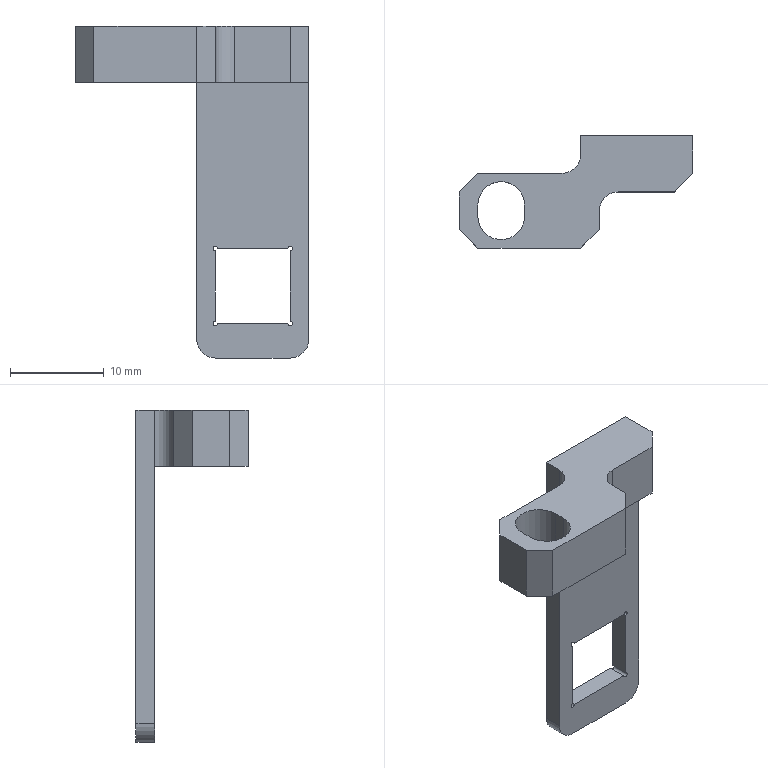Part | SolidWorks | features ICE 7, Fillet 2, 3DProfileFeature 1, Chamfer 1, Extrusion 1, HoleWzd 1 | 1 solid | 34 faces | box 25 x 12 x 35.5 mm | volume 1512 mm3 | plane 22 | cylinder 12 | commonest cylinder face diameters 0.5 x6 4 x4 5 x2
STEP:
#1=CARTESIAN_POINT('',(4.,0.,-9.8));
#2=VERTEX_POINT('',#1);
#3=CARTESIAN_POINT('',(4.,0.,-10.3));
#4=VERTEX_POINT('',#3);
#5=CARTESIAN_POINT('',(4.,0.,-10.05));
#6=DIRECTION('',(0.,1.,0.));
#7=DIRECTION('',(0.,0.,1.));
#8=AXIS2_PLACEMENT_3D('',#5,#6,#7);
#9=CIRCLE('',#8,0.25);
#10=EDGE_CURVE('',#2,#4,#9,.T.);
#11=ORIENTED_EDGE('',*,*,#10,.F.);
#12=CARTESIAN_POINT('',(4.,2.,-9.8));
#13=VERTEX_POINT('',#12);
#14=CARTESIAN_POINT('',(4.,-8.,-9.8));
#15=DIRECTION('',(0.,1.,0.));
#16=VECTOR('',#15,1000.);
#17=LINE('',#14,#16);
#18=EDGE_CURVE('',#2,#13,#17,.T.);
#19=ORIENTED_EDGE('',*,*,#18,.T.);
#20=CARTESIAN_POINT('',(4.,2.,-10.3));
#21=VERTEX_POINT('',#20);
#22=CARTESIAN_POINT('',(4.,2.,-10.05));
#23=DIRECTION('',(0.,1.,0.));
#24=DIRECTION('',(0.,0.,1.));
#25=AXIS2_PLACEMENT_3D('',#22,#23,#24);
#26=CIRCLE('',#25,0.25);
#27=EDGE_CURVE('',#13,#21,#26,.T.);
#28=ORIENTED_EDGE('',*,*,#27,.T.);
#29=CARTESIAN_POINT('',(4.,-8.,-10.3));
#30=DIRECTION('',(0.,1.,0.));
#31=VECTOR('',#30,1000.);
#32=LINE('',#29,#31);
#33=EDGE_CURVE('',#4,#21,#32,.T.);
#34=ORIENTED_EDGE('',*,*,#33,.F.);
#35=EDGE_LOOP('',(#11,#19,#28,#34));
#36=FACE_OUTER_BOUND('',#35,.T.);
#37=CARTESIAN_POINT('',(4.,-8.,-10.05));
#38=DIRECTION('',(0.,1.,0.));
#39=DIRECTION('',(0.,0.,1.));
#40=AXIS2_PLACEMENT_3D('',#37,#38,#39);
#41=CYLINDRICAL_SURFACE('',#40,0.25);
#42=ADVANCED_FACE('',(#36),#41,.F.);
#43=CARTESIAN_POINT('',(-4.,0.,-9.8));
#44=VERTEX_POINT('',#43);
#45=CARTESIAN_POINT('',(-3.75,0.,-10.05));
#46=VERTEX_POINT('',#45);
#47=CARTESIAN_POINT('',(-4.,0.,-10.05));
#48=DIRECTION('',(0.,1.,0.));
#49=DIRECTION('',(0.,0.,1.));
#50=AXIS2_PLACEMENT_3D('',#47,#48,#49);
#51=CIRCLE('',#50,0.25);
#52=EDGE_CURVE('',#44,#46,#51,.T.);
#53=ORIENTED_EDGE('',*,*,#52,.F.);
#54=CARTESIAN_POINT('',(-4.,2.,-9.8));
#55=VERTEX_POINT('',#54);
#56=CARTESIAN_POINT('',(-4.,-8.,-9.8));
#57=DIRECTION('',(0.,1.,0.));
#58=VECTOR('',#57,1000.);
#59=LINE('',#56,#58);
#60=EDGE_CURVE('',#44,#55,#59,.T.);
#61=ORIENTED_EDGE('',*,*,#60,.T.);
#62=CARTESIAN_POINT('',(-3.75,2.,-10.05));
#63=VERTEX_POINT('',#62);
#64=CARTESIAN_POINT('',(-4.,2.,-10.05));
#65=DIRECTION('',(0.,1.,0.));
#66=DIRECTION('',(0.,0.,1.));
#67=AXIS2_PLACEMENT_3D('',#64,#65,#66);
#68=CIRCLE('',#67,0.25);
#69=EDGE_CURVE('',#55,#63,#68,.T.);
#70=ORIENTED_EDGE('',*,*,#69,.T.);
#71=CARTESIAN_POINT('',(-3.75,-8.,-10.05));
#72=DIRECTION('',(0.,1.,0.));
#73=VECTOR('',#72,1000.);
#74=LINE('',#71,#73);
#75=EDGE_CURVE('',#46,#63,#74,.T.);
#76=ORIENTED_EDGE('',*,*,#75,.F.);
#77=EDGE_LOOP('',(#53,#61,#70,#76));
#78=FACE_OUTER_BOUND('',#77,.T.);
#79=CARTESIAN_POINT('',(-4.,-8.,-10.05));
#80=DIRECTION('',(0.,1.,0.));
#81=DIRECTION('',(0.,0.,1.));
#82=AXIS2_PLACEMENT_3D('',#79,#80,#81);
#83=CYLINDRICAL_SURFACE('',#82,0.25);
#84=ADVANCED_FACE('',(#78),#83,.F.);
#85=CARTESIAN_POINT('',(6.,0.,7.75));
#86=VERTEX_POINT('',#85);
#87=CARTESIAN_POINT('',(6.,0.,-19.75));
#88=VERTEX_POINT('',#87);
#89=CARTESIAN_POINT('',(6.,0.,-21.75));
#90=DIRECTION('',(0.,0.,-1.));
#91=VECTOR('',#90,1000.);
#92=LINE('',#89,#91);
#93=EDGE_CURVE('',#86,#88,#92,.T.);
#94=ORIENTED_EDGE('',*,*,#93,.T.);
#95=CARTESIAN_POINT('',(6.,2.,-19.75));
#96=VERTEX_POINT('',#95);
#97=CARTESIAN_POINT('',(6.,2.,-19.75));
#98=DIRECTION('',(0.,1.,0.));
#99=VECTOR('',#98,1000.);
#100=LINE('',#97,#99);
#101=EDGE_CURVE('',#88,#96,#100,.T.);
#102=ORIENTED_EDGE('',*,*,#101,.T.);
#103=CARTESIAN_POINT('',(6.,2.,13.75));
#104=VERTEX_POINT('',#103);
#105=CARTESIAN_POINT('',(6.,2.,-21.75));
#106=DIRECTION('',(0.,0.,-1.));
#107=VECTOR('',#106,1000.);
#108=LINE('',#105,#107);
#109=EDGE_CURVE('',#104,#96,#108,.T.);
#110=ORIENTED_EDGE('',*,*,#109,.F.);
#111=CARTESIAN_POINT('',(6.,-2.,13.75));
#112=VERTEX_POINT('',#111);
#113=CARTESIAN_POINT('',(6.,-10.,13.75));
#114=DIRECTION('',(0.,1.,0.));
#115=VECTOR('',#114,1000.);
#116=LINE('',#113,#115);
#117=EDGE_CURVE('',#112,#104,#116,.T.);
#118=ORIENTED_EDGE('',*,*,#117,.F.);
#119=CARTESIAN_POINT('',(6.,-2.,7.75));
#120=VERTEX_POINT('',#119);
#121=CARTESIAN_POINT('',(6.,-2.,-21.75));
#122=DIRECTION('',(0.,0.,-1.));
#123=VECTOR('',#122,1000.);
#124=LINE('',#121,#123);
#125=EDGE_CURVE('',#112,#120,#124,.T.);
#126=ORIENTED_EDGE('',*,*,#125,.T.);
#127=CARTESIAN_POINT('',(6.,2.,7.75));
#128=DIRECTION('',(0.,1.,0.));
#129=VECTOR('',#128,1000.);
#130=LINE('',#127,#129);
#131=EDGE_CURVE('',#120,#86,#130,.T.);
#132=ORIENTED_EDGE('',*,*,#131,.T.);
#133=EDGE_LOOP('',(#94,#102,#110,#118,#126,#132));
#134=FACE_OUTER_BOUND('',#133,.T.);
#135=CARTESIAN_POINT('',(6.,2.,-21.75));
#136=DIRECTION('',(-1.,0.,0.));
#137=DIRECTION('',(0.,0.,1.));
#138=AXIS2_PLACEMENT_3D('',#135,#136,#137);
#139=PLANE('',#138);
#140=ADVANCED_FACE('',(#134),#139,.F.);
#141=CARTESIAN_POINT('',(4.,2.,-21.75));
#142=VERTEX_POINT('',#141);
#143=CARTESIAN_POINT('',(-4.,2.,-21.75));
#144=VERTEX_POINT('',#143);
#145=CARTESIAN_POINT('',(-6.,2.,-21.75));
#146=DIRECTION('',(-1.,0.,0.));
#147=VECTOR('',#146,1000.);
#148=LINE('',#145,#147);
#149=EDGE_CURVE('',#142,#144,#148,.T.);
#150=ORIENTED_EDGE('',*,*,#149,.F.);
#151=CARTESIAN_POINT('',(4.,0.,-21.75));
#152=VERTEX_POINT('',#151);
#153=CARTESIAN_POINT('',(4.,2.,-21.75));
#154=DIRECTION('',(0.,-1.,0.));
#155=VECTOR('',#154,1000.);
#156=LINE('',#153,#155);
#157=EDGE_CURVE('',#142,#152,#156,.T.);
#158=ORIENTED_EDGE('',*,*,#157,.T.);
#159=CARTESIAN_POINT('',(-4.,0.,-21.75));
#160=VERTEX_POINT('',#159);
#161=CARTESIAN_POINT('',(-6.,0.,-21.75));
#162=DIRECTION('',(-1.,0.,0.));
#163=VECTOR('',#162,1000.);
#164=LINE('',#161,#163);
#165=EDGE_CURVE('',#152,#160,#164,.T.);
#166=ORIENTED_EDGE('',*,*,#165,.T.);
#167=CARTESIAN_POINT('',(-4.,2.,-21.75));
#168=DIRECTION('',(0.,1.,0.));
#169=VECTOR('',#168,1000.);
#170=LINE('',#167,#169);
#171=EDGE_CURVE('',#160,#144,#170,.T.);
#172=ORIENTED_EDGE('',*,*,#171,.T.);
#173=EDGE_LOOP('',(#150,#158,#166,#172));
#174=FACE_OUTER_BOUND('',#173,.T.);
#175=CARTESIAN_POINT('',(-6.,2.,-21.75));
#176=DIRECTION('',(0.,0.,1.));
#177=DIRECTION('',(1.,0.,0.));
#178=AXIS2_PLACEMENT_3D('',#175,#176,#177);
#179=PLANE('',#178);
#180=ADVANCED_FACE('',(#174),#179,.F.);
#181=CARTESIAN_POINT('',(-6.,2.,-19.75));
#182=VERTEX_POINT('',#181);
#183=CARTESIAN_POINT('',(-6.,2.,13.75));
#184=VERTEX_POINT('',#183);
#185=CARTESIAN_POINT('',(-6.,2.,-21.75));
#186=DIRECTION('',(0.,0.,1.));
#187=VECTOR('',#186,1000.);
#188=LINE('',#185,#187);
#189=EDGE_CURVE('',#182,#184,#188,.T.);
#190=ORIENTED_EDGE('',*,*,#189,.F.);
#191=CARTESIAN_POINT('',(-6.,0.,-19.75));
#192=VERTEX_POINT('',#191);
#193=CARTESIAN_POINT('',(-6.,2.,-19.75));
#194=DIRECTION('',(0.,-1.,0.));
#195=VECTOR('',#194,1000.);
#196=LINE('',#193,#195);
#197=EDGE_CURVE('',#182,#192,#196,.T.);
#198=ORIENTED_EDGE('',*,*,#197,.T.);
#199=CARTESIAN_POINT('',(-6.,0.,7.75));
#200=VERTEX_POINT('',#199);
#201=CARTESIAN_POINT('',(-6.,0.,-21.75));
#202=DIRECTION('',(0.,0.,1.));
#203=VECTOR('',#202,1000.);
#204=LINE('',#201,#203);
#205=EDGE_CURVE('',#192,#200,#204,.T.);
#206=ORIENTED_EDGE('',*,*,#205,.T.);
#207=CARTESIAN_POINT('',(-6.,0.,13.75));
#208=VERTEX_POINT('',#207);
#209=CARTESIAN_POINT('',(-6.,0.,13.75));
#210=DIRECTION('',(0.,0.,1.));
#211=VECTOR('',#210,1000.);
#212=LINE('',#209,#211);
#213=EDGE_CURVE('',#200,#208,#212,.T.);
#214=ORIENTED_EDGE('',*,*,#213,.T.);
#215=CARTESIAN_POINT('',(-6.,2.,13.75));
#216=DIRECTION('',(0.,1.,0.));
#217=VECTOR('',#216,1000.);
#218=LINE('',#215,#217);
#219=EDGE_CURVE('',#208,#184,#218,.T.);
#220=ORIENTED_EDGE('',*,*,#219,.T.);
#221=EDGE_LOOP('',(#190,#198,#206,#214,#220));
#222=FACE_OUTER_BOUND('',#221,.T.);
#223=CARTESIAN_POINT('',(-6.,2.,-21.75));
#224=DIRECTION('',(1.,0.,0.));
#225=DIRECTION('',(0.,0.,-1.));
#226=AXIS2_PLACEMENT_3D('',#223,#224,#225);
#227=PLANE('',#226);
#228=ADVANCED_FACE('',(#222),#227,.F.);
#229=CARTESIAN_POINT('',(4.,2.,-17.8));
#230=VERTEX_POINT('',#229);
#231=CARTESIAN_POINT('',(3.75,2.,-18.05));
#232=VERTEX_POINT('',#231);
#233=CARTESIAN_POINT('',(4.,2.,-18.05));
#234=DIRECTION('',(0.,1.,0.));
#235=DIRECTION('',(0.,0.,1.));
#236=AXIS2_PLACEMENT_3D('',#233,#234,#235);
#237=CIRCLE('',#236,0.25);
#238=EDGE_CURVE('',#230,#232,#237,.T.);
#239=ORIENTED_EDGE('',*,*,#238,.F.);
#240=CARTESIAN_POINT('',(4.,2.,-10.05));
#241=DIRECTION('',(0.,0.,-1.));
#242=VECTOR('',#241,1000.);
#243=LINE('',#240,#242);
#244=EDGE_CURVE('',#21,#230,#243,.T.);
#245=ORIENTED_EDGE('',*,*,#244,.F.);
#246=ORIENTED_EDGE('',*,*,#27,.F.);
#247=CARTESIAN_POINT('',(3.75,2.,-10.05));
#248=VERTEX_POINT('',#247);
#249=CARTESIAN_POINT('',(4.,2.,-10.05));
#250=DIRECTION('',(0.,1.,0.));
#251=DIRECTION('',(0.,0.,1.));
#252=AXIS2_PLACEMENT_3D('',#249,#250,#251);
#253=CIRCLE('',#252,0.25);
#254=EDGE_CURVE('',#248,#13,#253,.T.);
#255=ORIENTED_EDGE('',*,*,#254,.F.);
#256=CARTESIAN_POINT('',(-4.,2.,-10.05));
#257=DIRECTION('',(1.,0.,0.));
#258=VECTOR('',#257,1000.);
#259=LINE('',#256,#258);
#260=EDGE_CURVE('',#63,#248,#259,.T.);
#261=ORIENTED_EDGE('',*,*,#260,.F.);
#262=ORIENTED_EDGE('',*,*,#69,.F.);
#263=CARTESIAN_POINT('',(-4.,2.,-10.3));
#264=VERTEX_POINT('',#263);
#265=CARTESIAN_POINT('',(-4.,2.,-10.05));
#266=DIRECTION('',(0.,1.,0.));
#267=DIRECTION('',(0.,0.,1.));
#268=AXIS2_PLACEMENT_3D('',#265,#266,#267);
#269=CIRCLE('',#268,0.25);
#270=EDGE_CURVE('',#264,#55,#269,.T.);
#271=ORIENTED_EDGE('',*,*,#270,.F.);
#272=CARTESIAN_POINT('',(-4.,2.,-17.8));
#273=VERTEX_POINT('',#272);
#274=CARTESIAN_POINT('',(-4.,2.,-10.05));
#275=DIRECTION('',(0.,0.,1.));
#276=VECTOR('',#275,1000.);
#277=LINE('',#274,#276);
#278=EDGE_CURVE('',#273,#264,#277,.T.);
#279=ORIENTED_EDGE('',*,*,#278,.F.);
#280=CARTESIAN_POINT('',(-3.75,2.,-18.05));
#281=VERTEX_POINT('',#280);
#282=CARTESIAN_POINT('',(-4.,2.,-18.05));
#283=DIRECTION('',(0.,1.,0.));
#284=DIRECTION('',(0.,0.,1.));
#285=AXIS2_PLACEMENT_3D('',#282,#283,#284);
#286=CIRCLE('',#285,0.25);
#287=EDGE_CURVE('',#281,#273,#286,.T.);
#288=ORIENTED_EDGE('',*,*,#287,.F.);
#289=CARTESIAN_POINT('',(-4.,2.,-18.05));
#290=DIRECTION('',(-1.,0.,0.));
#291=VECTOR('',#290,1000.);
#292=LINE('',#289,#291);
#293=EDGE_CURVE('',#232,#281,#292,.T.);
#294=ORIENTED_EDGE('',*,*,#293,.F.);
#295=EDGE_LOOP('',(#239,#245,#246,#255,#261,#262,#271,#279,#288,#294));
#296=FACE_BOUND('',#295,.T.);
#297=ORIENTED_EDGE('',*,*,#109,.T.);
#298=CARTESIAN_POINT('',(4.,2.,-19.75));
#299=DIRECTION('',(0.,1.,0.));
#300=DIRECTION('',(0.,0.,1.));
#301=AXIS2_PLACEMENT_3D('',#298,#299,#300);
#302=CIRCLE('',#301,2.);
#303=EDGE_CURVE('',#96,#142,#302,.T.);
#304=ORIENTED_EDGE('',*,*,#303,.T.);
#305=ORIENTED_EDGE('',*,*,#149,.T.);
#306=CARTESIAN_POINT('',(-4.,2.,-19.75));
#307=DIRECTION('',(0.,1.,0.));
#308=DIRECTION('',(0.,0.,1.));
#309=AXIS2_PLACEMENT_3D('',#306,#307,#308);
#310=CIRCLE('',#309,2.);
#311=EDGE_CURVE('',#144,#182,#310,.T.);
#312=ORIENTED_EDGE('',*,*,#311,.T.);
#313=ORIENTED_EDGE('',*,*,#189,.T.);
#314=CARTESIAN_POINT('',(6.,2.,13.75));
#315=DIRECTION('',(-1.,0.,0.));
#316=VECTOR('',#315,1000.);
#317=LINE('',#314,#316);
#318=EDGE_CURVE('',#104,#184,#317,.T.);
#319=ORIENTED_EDGE('',*,*,#318,.F.);
#320=EDGE_LOOP('',(#297,#304,#305,#312,#313,#319));
#321=FACE_OUTER_BOUND('',#320,.T.);
#322=CARTESIAN_POINT('',(0.,2.,0.));
#323=DIRECTION('',(0.,1.,0.));
#324=DIRECTION('',(0.,0.,1.));
#325=AXIS2_PLACEMENT_3D('',#322,#323,#324);
#326=PLANE('',#325);
#327=ADVANCED_FACE('',(#296,#321),#326,.T.);
#328=CARTESIAN_POINT('',(4.,0.,-17.8));
#329=VERTEX_POINT('',#328);
#330=CARTESIAN_POINT('',(4.,0.,0.));
#331=DIRECTION('',(0.,0.,-1.));
#332=VECTOR('',#331,1000.);
#333=LINE('',#330,#332);
#334=EDGE_CURVE('',#4,#329,#333,.T.);
#335=ORIENTED_EDGE('',*,*,#334,.T.);
#336=CARTESIAN_POINT('',(3.75,0.,-18.05));
#337=VERTEX_POINT('',#336);
#338=CARTESIAN_POINT('',(4.,0.,-18.05));
#339=DIRECTION('',(0.,1.,0.));
#340=DIRECTION('',(0.,0.,1.));
#341=AXIS2_PLACEMENT_3D('',#338,#339,#340);
#342=CIRCLE('',#341,0.25);
#343=EDGE_CURVE('',#329,#337,#342,.T.);
#344=ORIENTED_EDGE('',*,*,#343,.T.);
#345=CARTESIAN_POINT('',(-3.75,0.,-18.05));
#346=VERTEX_POINT('',#345);
#347=CARTESIAN_POINT('',(0.,0.,-18.05));
#348=DIRECTION('',(-1.,0.,0.));
#349=VECTOR('',#348,1000.);
#350=LINE('',#347,#349);
#351=EDGE_CURVE('',#337,#346,#350,.T.);
#352=ORIENTED_EDGE('',*,*,#351,.T.);
#353=CARTESIAN_POINT('',(-4.,0.,-17.8));
#354=VERTEX_POINT('',#353);
#355=CARTESIAN_POINT('',(-4.,0.,-18.05));
#356=DIRECTION('',(0.,1.,0.));
#357=DIRECTION('',(0.,0.,1.));
#358=AXIS2_PLACEMENT_3D('',#355,#356,#357);
#359=CIRCLE('',#358,0.25);
#360=EDGE_CURVE('',#346,#354,#359,.T.);
#361=ORIENTED_EDGE('',*,*,#360,.T.);
#362=CARTESIAN_POINT('',(-4.,0.,-10.3));
#363=VERTEX_POINT('',#362);
#364=CARTESIAN_POINT('',(-4.,0.,0.));
#365=DIRECTION('',(0.,0.,1.));
#366=VECTOR('',#365,1000.);
#367=LINE('',#364,#366);
#368=EDGE_CURVE('',#354,#363,#367,.T.);
#369=ORIENTED_EDGE('',*,*,#368,.T.);
#370=CARTESIAN_POINT('',(-4.,0.,-10.05));
#371=DIRECTION('',(0.,1.,0.));
#372=DIRECTION('',(0.,0.,1.));
#373=AXIS2_PLACEMENT_3D('',#370,#371,#372);
#374=CIRCLE('',#373,0.25);
#375=EDGE_CURVE('',#363,#44,#374,.T.);
#376=ORIENTED_EDGE('',*,*,#375,.T.);
#377=ORIENTED_EDGE('',*,*,#52,.T.);
#378=CARTESIAN_POINT('',(3.75,0.,-10.05));
#379=VERTEX_POINT('',#378);
#380=CARTESIAN_POINT('',(0.,0.,-10.05));
#381=DIRECTION('',(1.,0.,0.));
#382=VECTOR('',#381,1000.);
#383=LINE('',#380,#382);
#384=EDGE_CURVE('',#46,#379,#383,.T.);
#385=ORIENTED_EDGE('',*,*,#384,.T.);
#386=CARTESIAN_POINT('',(4.,0.,-10.05));
#387=DIRECTION('',(0.,1.,0.));
#388=DIRECTION('',(0.,0.,1.));
#389=AXIS2_PLACEMENT_3D('',#386,#387,#388);
#390=CIRCLE('',#389,0.25);
#391=EDGE_CURVE('',#379,#2,#390,.T.);
#392=ORIENTED_EDGE('',*,*,#391,.T.);
#393=ORIENTED_EDGE('',*,*,#10,.T.);
#394=EDGE_LOOP('',(#335,#344,#352,#361,#369,#376,#377,#385,#392,#393));
#395=FACE_BOUND('',#394,.T.);
#396=ORIENTED_EDGE('',*,*,#165,.F.);
#397=CARTESIAN_POINT('',(4.,0.,-19.75));
#398=DIRECTION('',(0.,-1.,0.));
#399=DIRECTION('',(0.,0.,1.));
#400=AXIS2_PLACEMENT_3D('',#397,#398,#399);
#401=CIRCLE('',#400,2.);
#402=EDGE_CURVE('',#152,#88,#401,.T.);
#403=ORIENTED_EDGE('',*,*,#402,.T.);
#404=ORIENTED_EDGE('',*,*,#93,.F.);
#405=CARTESIAN_POINT('',(0.,0.,7.75));
#406=DIRECTION('',(-1.,0.,0.));
#407=VECTOR('',#406,1000.);
#408=LINE('',#405,#407);
#409=EDGE_CURVE('',#86,#200,#408,.T.);
#410=ORIENTED_EDGE('',*,*,#409,.T.);
#411=ORIENTED_EDGE('',*,*,#205,.F.);
#412=CARTESIAN_POINT('',(-4.,0.,-19.75));
#413=DIRECTION('',(0.,-1.,0.));
#414=DIRECTION('',(0.,0.,1.));
#415=AXIS2_PLACEMENT_3D('',#412,#413,#414);
#416=CIRCLE('',#415,2.);
#417=EDGE_CURVE('',#192,#160,#416,.T.);
#418=ORIENTED_EDGE('',*,*,#417,.T.);
#419=EDGE_LOOP('',(#396,#403,#404,#410,#411,#418));
#420=FACE_OUTER_BOUND('',#419,.T.);
#421=CARTESIAN_POINT('',(0.,0.,0.));
#422=DIRECTION('',(0.,1.,0.));
#423=DIRECTION('',(0.,0.,1.));
#424=AXIS2_PLACEMENT_3D('',#421,#422,#423);
#425=PLANE('',#424);
#426=ADVANCED_FACE('',(#395,#420),#425,.F.);
#427=CARTESIAN_POINT('',(-17.,-5.4,7.75));
#428=VERTEX_POINT('',#427);
#429=CARTESIAN_POINT('',(-12.,-5.4,7.75));
#430=VERTEX_POINT('',#429);
#431=CARTESIAN_POINT('',(-14.5,-5.4,7.75));
#432=DIRECTION('',(0.,0.,-1.));
#433=DIRECTION('',(-1.,0.,0.));
#434=AXIS2_PLACEMENT_3D('',#431,#432,#433);
#435=CIRCLE('',#434,2.5);
#436=EDGE_CURVE('',#428,#430,#435,.T.);
#437=ORIENTED_EDGE('',*,*,#436,.F.);
#438=CARTESIAN_POINT('',(-17.,-6.6,7.75));
#439=VERTEX_POINT('',#438);
#440=CARTESIAN_POINT('',(-17.,0.,7.75));
#441=DIRECTION('',(0.,1.,0.));
#442=VECTOR('',#441,1000.);
#443=LINE('',#440,#442);
#444=EDGE_CURVE('',#439,#428,#443,.T.);
#445=ORIENTED_EDGE('',*,*,#444,.F.);
#446=CARTESIAN_POINT('',(-12.,-6.6,7.75));
#447=VERTEX_POINT('',#446);
#448=CARTESIAN_POINT('',(-14.5,-6.6,7.75));
#449=DIRECTION('',(0.,0.,-1.));
#450=DIRECTION('',(-1.,0.,0.));
#451=AXIS2_PLACEMENT_3D('',#448,#449,#450);
#452=CIRCLE('',#451,2.5);
#453=EDGE_CURVE('',#447,#439,#452,.T.);
#454=ORIENTED_EDGE('',*,*,#453,.F.);
#455=CARTESIAN_POINT('',(-12.,0.,7.75));
#456=DIRECTION('',(0.,-1.,0.));
#457=VECTOR('',#456,1000.);
#458=LINE('',#455,#457);
#459=EDGE_CURVE('',#430,#447,#458,.T.);
#460=ORIENTED_EDGE('',*,*,#459,.F.);
#461=EDGE_LOOP('',(#437,#445,#454,#460));
#462=FACE_BOUND('',#461,.T.);
#463=ORIENTED_EDGE('',*,*,#131,.F.);
#464=CARTESIAN_POINT('',(4.,-4.,7.75));
#465=VERTEX_POINT('',#464);
#466=CARTESIAN_POINT('',(4.,-4.,7.75));
#467=DIRECTION('',(-0.7071,-0.7071,0.));
#468=VECTOR('',#467,1000.);
#469=LINE('',#466,#468);
#470=EDGE_CURVE('',#120,#465,#469,.T.);
#471=ORIENTED_EDGE('',*,*,#470,.T.);
#472=CARTESIAN_POINT('',(-2.,-4.,7.75));
#473=VERTEX_POINT('',#472);
#474=CARTESIAN_POINT('',(0.,-4.,7.75));
#475=DIRECTION('',(1.,0.,0.));
#476=VECTOR('',#475,1000.);
#477=LINE('',#474,#476);
#478=EDGE_CURVE('',#473,#465,#477,.T.);
#479=ORIENTED_EDGE('',*,*,#478,.F.);
#480=CARTESIAN_POINT('',(-4.,-6.,7.75));
#481=VERTEX_POINT('',#480);
#482=CARTESIAN_POINT('',(-2.,-6.,7.75));
#483=DIRECTION('',(0.,0.,1.));
#484=DIRECTION('',(-1.,0.,0.));
#485=AXIS2_PLACEMENT_3D('',#482,#483,#484);
#486=CIRCLE('',#485,2.);
#487=EDGE_CURVE('',#473,#481,#486,.T.);
#488=ORIENTED_EDGE('',*,*,#487,.T.);
#489=CARTESIAN_POINT('',(-4.,-8.,7.75));
#490=VERTEX_POINT('',#489);
#491=CARTESIAN_POINT('',(-4.,0.,7.75));
#492=DIRECTION('',(0.,1.,0.));
#493=VECTOR('',#492,1000.);
#494=LINE('',#491,#493);
#495=EDGE_CURVE('',#490,#481,#494,.T.);
#496=ORIENTED_EDGE('',*,*,#495,.F.);
#497=CARTESIAN_POINT('',(-6.,-10.,7.75));
#498=VERTEX_POINT('',#497);
#499=CARTESIAN_POINT('',(2.,-2.,7.75));
#500=DIRECTION('',(-0.7071,-0.7071,0.));
#501=VECTOR('',#500,1000.);
#502=LINE('',#499,#501);
#503=EDGE_CURVE('',#490,#498,#502,.T.);
#504=ORIENTED_EDGE('',*,*,#503,.T.);
#505=CARTESIAN_POINT('',(-17.,-10.,7.75));
#506=VERTEX_POINT('',#505);
#507=CARTESIAN_POINT('',(6.,-10.,7.75));
#508=DIRECTION('',(1.,0.,0.));
#509=VECTOR('',#508,1000.);
#510=LINE('',#507,#509);
#511=EDGE_CURVE('',#506,#498,#510,.T.);
#512=ORIENTED_EDGE('',*,*,#511,.F.);
#513=CARTESIAN_POINT('',(-19.,-8.,7.75));
#514=VERTEX_POINT('',#513);
#515=CARTESIAN_POINT('',(-13.5,-13.5,7.75));
#516=DIRECTION('',(-0.7071,0.7071,0.));
#517=VECTOR('',#516,1000.);
#518=LINE('',#515,#517);
#519=EDGE_CURVE('',#506,#514,#518,.T.);
#520=ORIENTED_EDGE('',*,*,#519,.T.);
#521=CARTESIAN_POINT('',(-19.,-4.,7.75));
#522=VERTEX_POINT('',#521);
#523=CARTESIAN_POINT('',(-19.,2.,7.75));
#524=DIRECTION('',(0.,-1.,0.));
#525=VECTOR('',#524,1000.);
#526=LINE('',#523,#525);
#527=EDGE_CURVE('',#522,#514,#526,.T.);
#528=ORIENTED_EDGE('',*,*,#527,.F.);
#529=CARTESIAN_POINT('',(-17.,-2.,7.75));
#530=VERTEX_POINT('',#529);
#531=CARTESIAN_POINT('',(-7.5,7.5,7.75));
#532=DIRECTION('',(0.7071,0.7071,0.));
#533=VECTOR('',#532,1000.);
#534=LINE('',#531,#533);
#535=EDGE_CURVE('',#522,#530,#534,.T.);
#536=ORIENTED_EDGE('',*,*,#535,.T.);
#537=CARTESIAN_POINT('',(-8.,-2.,7.75));
#538=VERTEX_POINT('',#537);
#539=CARTESIAN_POINT('',(0.,-2.,7.75));
#540=DIRECTION('',(-1.,0.,0.));
#541=VECTOR('',#540,1000.);
#542=LINE('',#539,#541);
#543=EDGE_CURVE('',#538,#530,#542,.T.);
#544=ORIENTED_EDGE('',*,*,#543,.F.);
#545=CARTESIAN_POINT('',(-8.,0.,7.75));
#546=DIRECTION('',(0.,0.,1.));
#547=DIRECTION('',(-1.,0.,0.));
#548=AXIS2_PLACEMENT_3D('',#545,#546,#547);
#549=CIRCLE('',#548,2.);
#550=EDGE_CURVE('',#538,#200,#549,.T.);
#551=ORIENTED_EDGE('',*,*,#550,.T.);
#552=ORIENTED_EDGE('',*,*,#409,.F.);
#553=EDGE_LOOP('',(#463,#471,#479,#488,#496,#504,#512,#520,#528,#536,#544,#551,#552));
#554=FACE_OUTER_BOUND('',#553,.T.);
#555=CARTESIAN_POINT('',(0.,0.,7.75));
#556=DIRECTION('',(0.,0.,-1.));
#557=DIRECTION('',(-1.,0.,0.));
#558=AXIS2_PLACEMENT_3D('',#555,#556,#557);
#559=PLANE('',#558);
#560=ADVANCED_FACE('',(#462,#554),#559,.T.);
#561=ORIENTED_EDGE('',*,*,#511,.T.);
#562=CARTESIAN_POINT('',(-6.,-10.,13.75));
#563=VERTEX_POINT('',#562);
#564=CARTESIAN_POINT('',(-6.,-10.,13.75));
#565=DIRECTION('',(0.,0.,1.));
#566=VECTOR('',#565,1000.);
#567=LINE('',#564,#566);
#568=EDGE_CURVE('',#498,#563,#567,.T.);
#569=ORIENTED_EDGE('',*,*,#568,.T.);
#570=CARTESIAN_POINT('',(-17.,-10.,13.75));
#571=VERTEX_POINT('',#570);
#572=CARTESIAN_POINT('',(6.,-10.,13.75));
#573=DIRECTION('',(-1.,0.,0.));
#574=VECTOR('',#573,1000.);
#575=LINE('',#572,#574);
#576=EDGE_CURVE('',#563,#571,#575,.T.);
#577=ORIENTED_EDGE('',*,*,#576,.T.);
#578=CARTESIAN_POINT('',(-17.,-10.,7.75));
#579=DIRECTION('',(0.,0.,-1.));
#580=VECTOR('',#579,1000.);
#581=LINE('',#578,#580);
#582=EDGE_CURVE('',#571,#506,#581,.T.);
#583=ORIENTED_EDGE('',*,*,#582,.T.);
#584=EDGE_LOOP('',(#561,#569,#577,#583));
#585=FACE_OUTER_BOUND('',#584,.T.);
#586=CARTESIAN_POINT('',(6.,-10.,7.75));
#587=DIRECTION('',(0.,-1.,0.));
#588=DIRECTION('',(1.,0.,0.));
#589=AXIS2_PLACEMENT_3D('',#586,#587,#588);
#590=PLANE('',#589);
#591=ADVANCED_FACE('',(#585),#590,.T.);
#592=ORIENTED_EDGE('',*,*,#527,.T.);
#593=CARTESIAN_POINT('',(-19.,-8.,13.75));
#594=VERTEX_POINT('',#593);
#595=CARTESIAN_POINT('',(-19.,-8.,7.75));
#596=DIRECTION('',(0.,0.,1.));
#597=VECTOR('',#596,1000.);
#598=LINE('',#595,#597);
#599=EDGE_CURVE('',#514,#594,#598,.T.);
#600=ORIENTED_EDGE('',*,*,#599,.T.);
#601=CARTESIAN_POINT('',(-19.,-4.,13.75));
#602=VERTEX_POINT('',#601);
#603=CARTESIAN_POINT('',(-19.,-10.,13.75));
#604=DIRECTION('',(0.,1.,0.));
#605=VECTOR('',#604,1000.);
#606=LINE('',#603,#605);
#607=EDGE_CURVE('',#594,#602,#606,.T.);
#608=ORIENTED_EDGE('',*,*,#607,.T.);
#609=CARTESIAN_POINT('',(-19.,-4.,7.75));
#610=DIRECTION('',(0.,0.,-1.));
#611=VECTOR('',#610,1000.);
#612=LINE('',#609,#611);
#613=EDGE_CURVE('',#602,#522,#612,.T.);
#614=ORIENTED_EDGE('',*,*,#613,.T.);
#615=EDGE_LOOP('',(#592,#600,#608,#614));
#616=FACE_OUTER_BOUND('',#615,.T.);
#617=CARTESIAN_POINT('',(-19.,2.,7.75));
#618=DIRECTION('',(-1.,0.,0.));
#619=DIRECTION('',(0.,-1.,0.));
#620=AXIS2_PLACEMENT_3D('',#617,#618,#619);
#621=PLANE('',#620);
#622=ADVANCED_FACE('',(#616),#621,.T.);
#623=CARTESIAN_POINT('',(-17.,-5.4,13.75));
#624=VERTEX_POINT('',#623);
#625=CARTESIAN_POINT('',(-17.,-6.6,13.75));
#626=VERTEX_POINT('',#625);
#627=CARTESIAN_POINT('',(-17.,-5.4,13.75));
#628=DIRECTION('',(0.,-1.,0.));
#629=VECTOR('',#628,1000.);
#630=LINE('',#627,#629);
#631=EDGE_CURVE('',#624,#626,#630,.T.);
#632=ORIENTED_EDGE('',*,*,#631,.F.);
#633=CARTESIAN_POINT('',(-12.,-5.4,13.75));
#634=VERTEX_POINT('',#633);
#635=CARTESIAN_POINT('',(-14.5,-5.4,13.75));
#636=DIRECTION('',(0.,0.,1.));
#637=DIRECTION('',(1.,0.,0.));
#638=AXIS2_PLACEMENT_3D('',#635,#636,#637);
#639=CIRCLE('',#638,2.5);
#640=EDGE_CURVE('',#634,#624,#639,.T.);
#641=ORIENTED_EDGE('',*,*,#640,.F.);
#642=CARTESIAN_POINT('',(-12.,-6.6,13.75));
#643=VERTEX_POINT('',#642);
#644=CARTESIAN_POINT('',(-12.,-5.4,13.75));
#645=DIRECTION('',(0.,1.,0.));
#646=VECTOR('',#645,1000.);
#647=LINE('',#644,#646);
#648=EDGE_CURVE('',#643,#634,#647,.T.);
#649=ORIENTED_EDGE('',*,*,#648,.F.);
#650=CARTESIAN_POINT('',(-14.5,-6.6,13.75));
#651=DIRECTION('',(0.,0.,1.));
#652=DIRECTION('',(1.,0.,0.));
#653=AXIS2_PLACEMENT_3D('',#650,#651,#652);
#654=CIRCLE('',#653,2.5);
#655=EDGE_CURVE('',#626,#643,#654,.T.);
#656=ORIENTED_EDGE('',*,*,#655,.F.);
#657=EDGE_LOOP('',(#632,#641,#649,#656));
#658=FACE_BOUND('',#657,.T.);
#659=CARTESIAN_POINT('',(4.,-4.,13.75));
#660=VERTEX_POINT('',#659);
#661=CARTESIAN_POINT('',(-2.,-4.,13.75));
#662=VERTEX_POINT('',#661);
#663=CARTESIAN_POINT('',(6.,-4.,13.75));
#664=DIRECTION('',(-1.,0.,0.));
#665=VECTOR('',#664,1000.);
#666=LINE('',#663,#665);
#667=EDGE_CURVE('',#660,#662,#666,.T.);
#668=ORIENTED_EDGE('',*,*,#667,.F.);
#669=CARTESIAN_POINT('',(4.,-4.,13.75));
#670=DIRECTION('',(0.7071,0.7071,0.));
#671=VECTOR('',#670,1000.);
#672=LINE('',#669,#671);
#673=EDGE_CURVE('',#660,#112,#672,.T.);
#674=ORIENTED_EDGE('',*,*,#673,.T.);
#675=ORIENTED_EDGE('',*,*,#117,.T.);
#676=ORIENTED_EDGE('',*,*,#318,.T.);
#677=ORIENTED_EDGE('',*,*,#219,.F.);
#678=CARTESIAN_POINT('',(-8.,-2.,13.75));
#679=VERTEX_POINT('',#678);
#680=CARTESIAN_POINT('',(-8.,0.,13.75));
#681=DIRECTION('',(0.,0.,-1.));
#682=DIRECTION('',(-1.,0.,0.));
#683=AXIS2_PLACEMENT_3D('',#680,#681,#682);
#684=CIRCLE('',#683,2.);
#685=EDGE_CURVE('',#208,#679,#684,.T.);
#686=ORIENTED_EDGE('',*,*,#685,.T.);
#687=CARTESIAN_POINT('',(-17.,-2.,13.75));
#688=VERTEX_POINT('',#687);
#689=CARTESIAN_POINT('',(-6.,-2.,13.75));
#690=DIRECTION('',(1.,0.,0.));
#691=VECTOR('',#690,1000.);
#692=LINE('',#689,#691);
#693=EDGE_CURVE('',#688,#679,#692,.T.);
#694=ORIENTED_EDGE('',*,*,#693,.F.);
#695=CARTESIAN_POINT('',(-17.,-2.,13.75));
#696=DIRECTION('',(-0.7071,-0.7071,0.));
#697=VECTOR('',#696,1000.);
#698=LINE('',#695,#697);
#699=EDGE_CURVE('',#688,#602,#698,.T.);
#700=ORIENTED_EDGE('',*,*,#699,.T.);
#701=ORIENTED_EDGE('',*,*,#607,.F.);
#702=CARTESIAN_POINT('',(-19.,-8.,13.75));
#703=DIRECTION('',(0.7071,-0.7071,0.));
#704=VECTOR('',#703,1000.);
#705=LINE('',#702,#704);
#706=EDGE_CURVE('',#594,#571,#705,.T.);
#707=ORIENTED_EDGE('',*,*,#706,.T.);
#708=ORIENTED_EDGE('',*,*,#576,.F.);
#709=CARTESIAN_POINT('',(-4.,-8.,13.75));
#710=VERTEX_POINT('',#709);
#711=CARTESIAN_POINT('',(-6.,-10.,13.75));
#712=DIRECTION('',(0.7071,0.7071,0.));
#713=VECTOR('',#712,1000.);
#714=LINE('',#711,#713);
#715=EDGE_CURVE('',#563,#710,#714,.T.);
#716=ORIENTED_EDGE('',*,*,#715,.T.);
#717=CARTESIAN_POINT('',(-4.,-6.,13.75));
#718=VERTEX_POINT('',#717);
#719=CARTESIAN_POINT('',(-4.,-10.,13.75));
#720=DIRECTION('',(0.,-1.,0.));
#721=VECTOR('',#720,1000.);
#722=LINE('',#719,#721);
#723=EDGE_CURVE('',#718,#710,#722,.T.);
#724=ORIENTED_EDGE('',*,*,#723,.F.);
#725=CARTESIAN_POINT('',(-2.,-6.,13.75));
#726=DIRECTION('',(0.,0.,-1.));
#727=DIRECTION('',(-1.,0.,0.));
#728=AXIS2_PLACEMENT_3D('',#725,#726,#727);
#729=CIRCLE('',#728,2.);
#730=EDGE_CURVE('',#718,#662,#729,.T.);
#731=ORIENTED_EDGE('',*,*,#730,.T.);
#732=EDGE_LOOP('',(#668,#674,#675,#676,#677,#686,#694,#700,#701,#707,#708,#716,#724,#731));
#733=FACE_OUTER_BOUND('',#732,.T.);
#734=CARTESIAN_POINT('',(6.,-10.,13.75));
#735=DIRECTION('',(0.,0.,-1.));
#736=DIRECTION('',(-1.,0.,0.));
#737=AXIS2_PLACEMENT_3D('',#734,#735,#736);
#738=PLANE('',#737);
#739=ADVANCED_FACE('',(#658,#733),#738,.F.);
#740=ORIENTED_EDGE('',*,*,#693,.T.);
#741=CARTESIAN_POINT('',(-8.,-2.,7.75));
#742=DIRECTION('',(0.,0.,-1.));
#743=VECTOR('',#742,1000.);
#744=LINE('',#741,#743);
#745=EDGE_CURVE('',#679,#538,#744,.T.);
#746=ORIENTED_EDGE('',*,*,#745,.T.);
#747=ORIENTED_EDGE('',*,*,#543,.T.);
#748=CARTESIAN_POINT('',(-17.,-2.,13.75));
#749=DIRECTION('',(0.,0.,1.));
#750=VECTOR('',#749,1000.);
#751=LINE('',#748,#750);
#752=EDGE_CURVE('',#530,#688,#751,.T.);
#753=ORIENTED_EDGE('',*,*,#752,.T.);
#754=EDGE_LOOP('',(#740,#746,#747,#753));
#755=FACE_OUTER_BOUND('',#754,.T.);
#756=CARTESIAN_POINT('',(-6.,-2.,-4.25));
#757=DIRECTION('',(0.,-1.,0.));
#758=DIRECTION('',(1.,0.,0.));
#759=AXIS2_PLACEMENT_3D('',#756,#757,#758);
#760=PLANE('',#759);
#761=ADVANCED_FACE('',(#755),#760,.F.);
#762=ORIENTED_EDGE('',*,*,#495,.T.);
#763=CARTESIAN_POINT('',(-4.,-6.,13.75));
#764=DIRECTION('',(0.,0.,1.));
#765=VECTOR('',#764,1000.);
#766=LINE('',#763,#765);
#767=EDGE_CURVE('',#481,#718,#766,.T.);
#768=ORIENTED_EDGE('',*,*,#767,.T.);
#769=ORIENTED_EDGE('',*,*,#723,.T.);
#770=CARTESIAN_POINT('',(-4.,-8.,7.75));
#771=DIRECTION('',(0.,0.,-1.));
#772=VECTOR('',#771,1000.);
#773=LINE('',#770,#772);
#774=EDGE_CURVE('',#710,#490,#773,.T.);
#775=ORIENTED_EDGE('',*,*,#774,.T.);
#776=EDGE_LOOP('',(#762,#768,#769,#775));
#777=FACE_OUTER_BOUND('',#776,.T.);
#778=CARTESIAN_POINT('',(-4.,-10.,-4.25));
#779=DIRECTION('',(-1.,0.,0.));
#780=DIRECTION('',(0.,0.,1.));
#781=AXIS2_PLACEMENT_3D('',#778,#779,#780);
#782=PLANE('',#781);
#783=ADVANCED_FACE('',(#777),#782,.F.);
#784=ORIENTED_EDGE('',*,*,#667,.T.);
#785=CARTESIAN_POINT('',(-2.,-4.,7.75));
#786=DIRECTION('',(0.,0.,-1.));
#787=VECTOR('',#786,1000.);
#788=LINE('',#785,#787);
#789=EDGE_CURVE('',#662,#473,#788,.T.);
#790=ORIENTED_EDGE('',*,*,#789,.T.);
#791=ORIENTED_EDGE('',*,*,#478,.T.);
#792=CARTESIAN_POINT('',(4.,-4.,-4.25));
#793=DIRECTION('',(0.,0.,1.));
#794=VECTOR('',#793,1000.);
#795=LINE('',#792,#794);
#796=EDGE_CURVE('',#465,#660,#795,.T.);
#797=ORIENTED_EDGE('',*,*,#796,.T.);
#798=EDGE_LOOP('',(#784,#790,#791,#797));
#799=FACE_OUTER_BOUND('',#798,.T.);
#800=CARTESIAN_POINT('',(6.,-4.,-4.25));
#801=DIRECTION('',(0.,1.,0.));
#802=DIRECTION('',(-1.,0.,0.));
#803=AXIS2_PLACEMENT_3D('',#800,#801,#802);
#804=PLANE('',#803);
#805=ADVANCED_FACE('',(#799),#804,.F.);
#806=ORIENTED_EDGE('',*,*,#470,.F.);
#807=ORIENTED_EDGE('',*,*,#125,.F.);
#808=ORIENTED_EDGE('',*,*,#673,.F.);
#809=ORIENTED_EDGE('',*,*,#796,.F.);
#810=EDGE_LOOP('',(#806,#807,#808,#809));
#811=FACE_OUTER_BOUND('',#810,.T.);
#812=CARTESIAN_POINT('',(4.,-4.,-4.25));
#813=DIRECTION('',(-0.7071,0.7071,0.));
#814=DIRECTION('',(0.,0.,1.));
#815=AXIS2_PLACEMENT_3D('',#812,#813,#814);
#816=PLANE('',#815);
#817=ADVANCED_FACE('',(#811),#816,.F.);
#818=ORIENTED_EDGE('',*,*,#503,.F.);
#819=ORIENTED_EDGE('',*,*,#774,.F.);
#820=ORIENTED_EDGE('',*,*,#715,.F.);
#821=ORIENTED_EDGE('',*,*,#568,.F.);
#822=EDGE_LOOP('',(#818,#819,#820,#821));
#823=FACE_OUTER_BOUND('',#822,.T.);
#824=CARTESIAN_POINT('',(-6.,-10.,7.75));
#825=DIRECTION('',(0.7071,-0.7071,0.));
#826=DIRECTION('',(0.,0.,-1.));
#827=AXIS2_PLACEMENT_3D('',#824,#825,#826);
#828=PLANE('',#827);
#829=ADVANCED_FACE('',(#823),#828,.T.);
#830=ORIENTED_EDGE('',*,*,#519,.F.);
#831=ORIENTED_EDGE('',*,*,#582,.F.);
#832=ORIENTED_EDGE('',*,*,#706,.F.);
#833=ORIENTED_EDGE('',*,*,#599,.F.);
#834=EDGE_LOOP('',(#830,#831,#832,#833));
#835=FACE_OUTER_BOUND('',#834,.T.);
#836=CARTESIAN_POINT('',(-19.,-8.,7.75));
#837=DIRECTION('',(0.7071,0.7071,0.));
#838=DIRECTION('',(0.,0.,1.));
#839=AXIS2_PLACEMENT_3D('',#836,#837,#838);
#840=PLANE('',#839);
#841=ADVANCED_FACE('',(#835),#840,.F.);
#842=ORIENTED_EDGE('',*,*,#535,.F.);
#843=ORIENTED_EDGE('',*,*,#613,.F.);
#844=ORIENTED_EDGE('',*,*,#699,.F.);
#845=ORIENTED_EDGE('',*,*,#752,.F.);
#846=EDGE_LOOP('',(#842,#843,#844,#845));
#847=FACE_OUTER_BOUND('',#846,.T.);
#848=CARTESIAN_POINT('',(-17.,-2.,-4.25));
#849=DIRECTION('',(-0.7071,0.7071,0.));
#850=DIRECTION('',(0.,0.,-1.));
#851=AXIS2_PLACEMENT_3D('',#848,#849,#850);
#852=PLANE('',#851);
#853=ADVANCED_FACE('',(#847),#852,.T.);
#854=ORIENTED_EDGE('',*,*,#487,.F.);
#855=ORIENTED_EDGE('',*,*,#789,.F.);
#856=ORIENTED_EDGE('',*,*,#730,.F.);
#857=ORIENTED_EDGE('',*,*,#767,.F.);
#858=EDGE_LOOP('',(#854,#855,#856,#857));
#859=FACE_OUTER_BOUND('',#858,.T.);
#860=CARTESIAN_POINT('',(-2.,-6.,-4.25));
#861=DIRECTION('',(0.,0.,-1.));
#862=DIRECTION('',(-1.,0.,0.));
#863=AXIS2_PLACEMENT_3D('',#860,#861,#862);
#864=CYLINDRICAL_SURFACE('',#863,2.);
#865=ADVANCED_FACE('',(#859),#864,.F.);
#866=ORIENTED_EDGE('',*,*,#550,.F.);
#867=ORIENTED_EDGE('',*,*,#745,.F.);
#868=ORIENTED_EDGE('',*,*,#685,.F.);
#869=ORIENTED_EDGE('',*,*,#213,.F.);
#870=EDGE_LOOP('',(#866,#867,#868,#869));
#871=FACE_OUTER_BOUND('',#870,.T.);
#872=CARTESIAN_POINT('',(-8.,0.,-21.75));
#873=DIRECTION('',(0.,0.,-1.));
#874=DIRECTION('',(-1.,0.,0.));
#875=AXIS2_PLACEMENT_3D('',#872,#873,#874);
#876=CYLINDRICAL_SURFACE('',#875,2.);
#877=ADVANCED_FACE('',(#871),#876,.F.);
#878=ORIENTED_EDGE('',*,*,#303,.F.);
#879=ORIENTED_EDGE('',*,*,#101,.F.);
#880=ORIENTED_EDGE('',*,*,#402,.F.);
#881=ORIENTED_EDGE('',*,*,#157,.F.);
#882=EDGE_LOOP('',(#878,#879,#880,#881));
#883=FACE_OUTER_BOUND('',#882,.T.);
#884=CARTESIAN_POINT('',(4.,2.,-19.75));
#885=DIRECTION('',(0.,-1.,0.));
#886=DIRECTION('',(0.,0.,-1.));
#887=AXIS2_PLACEMENT_3D('',#884,#885,#886);
#888=CYLINDRICAL_SURFACE('',#887,2.);
#889=ADVANCED_FACE('',(#883),#888,.T.);
#890=ORIENTED_EDGE('',*,*,#311,.F.);
#891=ORIENTED_EDGE('',*,*,#171,.F.);
#892=ORIENTED_EDGE('',*,*,#417,.F.);
#893=ORIENTED_EDGE('',*,*,#197,.F.);
#894=EDGE_LOOP('',(#890,#891,#892,#893));
#895=FACE_OUTER_BOUND('',#894,.T.);
#896=CARTESIAN_POINT('',(-4.,2.,-19.75));
#897=DIRECTION('',(0.,-1.,0.));
#898=DIRECTION('',(0.,0.,-1.));
#899=AXIS2_PLACEMENT_3D('',#896,#897,#898);
#900=CYLINDRICAL_SURFACE('',#899,2.);
#901=ADVANCED_FACE('',(#895),#900,.T.);
#902=ORIENTED_EDGE('',*,*,#244,.T.);
#903=CARTESIAN_POINT('',(4.,-8.,-17.8));
#904=DIRECTION('',(0.,-1.,0.));
#905=VECTOR('',#904,1000.);
#906=LINE('',#903,#905);
#907=EDGE_CURVE('',#230,#329,#906,.T.);
#908=ORIENTED_EDGE('',*,*,#907,.T.);
#909=ORIENTED_EDGE('',*,*,#334,.F.);
#910=ORIENTED_EDGE('',*,*,#33,.T.);
#911=EDGE_LOOP('',(#902,#908,#909,#910));
#912=FACE_OUTER_BOUND('',#911,.T.);
#913=CARTESIAN_POINT('',(4.,-8.,-10.05));
#914=DIRECTION('',(1.,0.,0.));
#915=DIRECTION('',(0.,0.,-1.));
#916=AXIS2_PLACEMENT_3D('',#913,#914,#915);
#917=PLANE('',#916);
#918=ADVANCED_FACE('',(#912),#917,.F.);
#919=ORIENTED_EDGE('',*,*,#260,.T.);
#920=CARTESIAN_POINT('',(3.75,-8.,-10.05));
#921=DIRECTION('',(0.,-1.,0.));
#922=VECTOR('',#921,1000.);
#923=LINE('',#920,#922);
#924=EDGE_CURVE('',#248,#379,#923,.T.);
#925=ORIENTED_EDGE('',*,*,#924,.T.);
#926=ORIENTED_EDGE('',*,*,#384,.F.);
#927=ORIENTED_EDGE('',*,*,#75,.T.);
#928=EDGE_LOOP('',(#919,#925,#926,#927));
#929=FACE_OUTER_BOUND('',#928,.T.);
#930=CARTESIAN_POINT('',(-4.,-8.,-10.05));
#931=DIRECTION('',(0.,0.,1.));
#932=DIRECTION('',(1.,0.,0.));
#933=AXIS2_PLACEMENT_3D('',#930,#931,#932);
#934=PLANE('',#933);
#935=ADVANCED_FACE('',(#929),#934,.F.);
#936=ORIENTED_EDGE('',*,*,#368,.F.);
#937=CARTESIAN_POINT('',(-4.,-8.,-17.8));
#938=DIRECTION('',(0.,1.,0.));
#939=VECTOR('',#938,1000.);
#940=LINE('',#937,#939);
#941=EDGE_CURVE('',#354,#273,#940,.T.);
#942=ORIENTED_EDGE('',*,*,#941,.T.);
#943=ORIENTED_EDGE('',*,*,#278,.T.);
#944=CARTESIAN_POINT('',(-4.,-8.,-10.3));
#945=DIRECTION('',(0.,-1.,0.));
#946=VECTOR('',#945,1000.);
#947=LINE('',#944,#946);
#948=EDGE_CURVE('',#264,#363,#947,.T.);
#949=ORIENTED_EDGE('',*,*,#948,.T.);
#950=EDGE_LOOP('',(#936,#942,#943,#949));
#951=FACE_OUTER_BOUND('',#950,.T.);
#952=CARTESIAN_POINT('',(-4.,-8.,-10.05));
#953=DIRECTION('',(-1.,0.,0.));
#954=DIRECTION('',(0.,0.,1.));
#955=AXIS2_PLACEMENT_3D('',#952,#953,#954);
#956=PLANE('',#955);
#957=ADVANCED_FACE('',(#951),#956,.F.);
#958=ORIENTED_EDGE('',*,*,#351,.F.);
#959=CARTESIAN_POINT('',(3.75,-8.,-18.05));
#960=DIRECTION('',(0.,1.,0.));
#961=VECTOR('',#960,1000.);
#962=LINE('',#959,#961);
#963=EDGE_CURVE('',#337,#232,#962,.T.);
#964=ORIENTED_EDGE('',*,*,#963,.T.);
#965=ORIENTED_EDGE('',*,*,#293,.T.);
#966=CARTESIAN_POINT('',(-3.75,-8.,-18.05));
#967=DIRECTION('',(0.,-1.,0.));
#968=VECTOR('',#967,1000.);
#969=LINE('',#966,#968);
#970=EDGE_CURVE('',#281,#346,#969,.T.);
#971=ORIENTED_EDGE('',*,*,#970,.T.);
#972=EDGE_LOOP('',(#958,#964,#965,#971));
#973=FACE_OUTER_BOUND('',#972,.T.);
#974=CARTESIAN_POINT('',(-4.,-8.,-18.05));
#975=DIRECTION('',(0.,0.,-1.));
#976=DIRECTION('',(-1.,0.,0.));
#977=AXIS2_PLACEMENT_3D('',#974,#975,#976);
#978=PLANE('',#977);
#979=ADVANCED_FACE('',(#973),#978,.F.);
#980=ORIENTED_EDGE('',*,*,#60,.F.);
#981=ORIENTED_EDGE('',*,*,#375,.F.);
#982=ORIENTED_EDGE('',*,*,#948,.F.);
#983=ORIENTED_EDGE('',*,*,#270,.T.);
#984=EDGE_LOOP('',(#980,#981,#982,#983));
#985=FACE_OUTER_BOUND('',#984,.T.);
#986=CARTESIAN_POINT('',(-4.,-8.,-10.05));
#987=DIRECTION('',(0.,1.,0.));
#988=DIRECTION('',(0.,0.,1.));
#989=AXIS2_PLACEMENT_3D('',#986,#987,#988);
#990=CYLINDRICAL_SURFACE('',#989,0.25);
#991=ADVANCED_FACE('',(#985),#990,.F.);
#992=ORIENTED_EDGE('',*,*,#18,.F.);
#993=ORIENTED_EDGE('',*,*,#391,.F.);
#994=ORIENTED_EDGE('',*,*,#924,.F.);
#995=ORIENTED_EDGE('',*,*,#254,.T.);
#996=EDGE_LOOP('',(#992,#993,#994,#995));
#997=FACE_OUTER_BOUND('',#996,.T.);
#998=CARTESIAN_POINT('',(4.,-8.,-10.05));
#999=DIRECTION('',(0.,1.,0.));
#1000=DIRECTION('',(0.,0.,1.));
#1001=AXIS2_PLACEMENT_3D('',#998,#999,#1000);
#1002=CYLINDRICAL_SURFACE('',#1001,0.25);
#1003=ADVANCED_FACE('',(#997),#1002,.F.);
#1004=ORIENTED_EDGE('',*,*,#360,.F.);
#1005=ORIENTED_EDGE('',*,*,#970,.F.);
#1006=ORIENTED_EDGE('',*,*,#287,.T.);
#1007=ORIENTED_EDGE('',*,*,#941,.F.);
#1008=EDGE_LOOP('',(#1004,#1005,#1006,#1007));
#1009=FACE_OUTER_BOUND('',#1008,.T.);
#1010=CARTESIAN_POINT('',(-4.,-8.,-18.05));
#1011=DIRECTION('',(0.,1.,0.));
#1012=DIRECTION('',(0.,0.,1.));
#1013=AXIS2_PLACEMENT_3D('',#1010,#1011,#1012);
#1014=CYLINDRICAL_SURFACE('',#1013,0.25);
#1015=ADVANCED_FACE('',(#1009),#1014,.F.);
#1016=ORIENTED_EDGE('',*,*,#238,.T.);
#1017=ORIENTED_EDGE('',*,*,#963,.F.);
#1018=ORIENTED_EDGE('',*,*,#343,.F.);
#1019=ORIENTED_EDGE('',*,*,#907,.F.);
#1020=EDGE_LOOP('',(#1016,#1017,#1018,#1019));
#1021=FACE_OUTER_BOUND('',#1020,.T.);
#1022=CARTESIAN_POINT('',(4.,-8.,-18.05));
#1023=DIRECTION('',(0.,1.,0.));
#1024=DIRECTION('',(0.,0.,1.));
#1025=AXIS2_PLACEMENT_3D('',#1022,#1023,#1024);
#1026=CYLINDRICAL_SURFACE('',#1025,0.25);
#1027=ADVANCED_FACE('',(#1021),#1026,.F.);
#1028=ORIENTED_EDGE('',*,*,#459,.T.);
#1029=CARTESIAN_POINT('',(-12.,-6.6,3.75));
#1030=DIRECTION('',(0.,0.,1.));
#1031=VECTOR('',#1030,1000.);
#1032=LINE('',#1029,#1031);
#1033=EDGE_CURVE('',#447,#643,#1032,.T.);
#1034=ORIENTED_EDGE('',*,*,#1033,.T.);
#1035=ORIENTED_EDGE('',*,*,#648,.T.);
#1036=CARTESIAN_POINT('',(-12.,-5.4,3.75));
#1037=DIRECTION('',(0.,0.,1.));
#1038=VECTOR('',#1037,1000.);
#1039=LINE('',#1036,#1038);
#1040=EDGE_CURVE('',#430,#634,#1039,.T.);
#1041=ORIENTED_EDGE('',*,*,#1040,.F.);
#1042=EDGE_LOOP('',(#1028,#1034,#1035,#1041));
#1043=FACE_OUTER_BOUND('',#1042,.T.);
#1044=CARTESIAN_POINT('',(-12.,-5.4,3.75));
#1045=DIRECTION('',(1.,0.,0.));
#1046=DIRECTION('',(0.,0.,-1.));
#1047=AXIS2_PLACEMENT_3D('',#1044,#1045,#1046);
#1048=PLANE('',#1047);
#1049=ADVANCED_FACE('',(#1043),#1048,.F.);
#1050=ORIENTED_EDGE('',*,*,#444,.T.);
#1051=CARTESIAN_POINT('',(-17.,-5.4,3.75));
#1052=DIRECTION('',(0.,0.,1.));
#1053=VECTOR('',#1052,1000.);
#1054=LINE('',#1051,#1053);
#1055=EDGE_CURVE('',#428,#624,#1054,.T.);
#1056=ORIENTED_EDGE('',*,*,#1055,.T.);
#1057=ORIENTED_EDGE('',*,*,#631,.T.);
#1058=CARTESIAN_POINT('',(-17.,-6.6,3.75));
#1059=DIRECTION('',(0.,0.,1.));
#1060=VECTOR('',#1059,1000.);
#1061=LINE('',#1058,#1060);
#1062=EDGE_CURVE('',#439,#626,#1061,.T.);
#1063=ORIENTED_EDGE('',*,*,#1062,.F.);
#1064=EDGE_LOOP('',(#1050,#1056,#1057,#1063));
#1065=FACE_OUTER_BOUND('',#1064,.T.);
#1066=CARTESIAN_POINT('',(-17.,-5.4,3.75));
#1067=DIRECTION('',(-1.,0.,0.));
#1068=DIRECTION('',(0.,0.,1.));
#1069=AXIS2_PLACEMENT_3D('',#1066,#1067,#1068);
#1070=PLANE('',#1069);
#1071=ADVANCED_FACE('',(#1065),#1070,.F.);
#1072=ORIENTED_EDGE('',*,*,#436,.T.);
#1073=ORIENTED_EDGE('',*,*,#1040,.T.);
#1074=ORIENTED_EDGE('',*,*,#640,.T.);
#1075=ORIENTED_EDGE('',*,*,#1055,.F.);
#1076=EDGE_LOOP('',(#1072,#1073,#1074,#1075));
#1077=FACE_OUTER_BOUND('',#1076,.T.);
#1078=CARTESIAN_POINT('',(-14.5,-5.4,3.75));
#1079=DIRECTION('',(0.,0.,1.));
#1080=DIRECTION('',(1.,0.,0.));
#1081=AXIS2_PLACEMENT_3D('',#1078,#1079,#1080);
#1082=CYLINDRICAL_SURFACE('',#1081,2.5);
#1083=ADVANCED_FACE('',(#1077),#1082,.F.);
#1084=ORIENTED_EDGE('',*,*,#453,.T.);
#1085=ORIENTED_EDGE('',*,*,#1062,.T.);
#1086=ORIENTED_EDGE('',*,*,#655,.T.);
#1087=ORIENTED_EDGE('',*,*,#1033,.F.);
#1088=EDGE_LOOP('',(#1084,#1085,#1086,#1087));
#1089=FACE_OUTER_BOUND('',#1088,.T.);
#1090=CARTESIAN_POINT('',(-14.5,-6.6,3.75));
#1091=DIRECTION('',(0.,0.,1.));
#1092=DIRECTION('',(1.,0.,0.));
#1093=AXIS2_PLACEMENT_3D('',#1090,#1091,#1092);
#1094=CYLINDRICAL_SURFACE('',#1093,2.5);
#1095=ADVANCED_FACE('',(#1089),#1094,.F.);
#1096=CLOSED_SHELL('',(#42,#84,#140,#180,#228,#327,#426,#560,#591,#622,#739,#761,#783,#805,#817,#829,#841,#853,#865,#877,#889,#901,#918,#935,#957,#979,#991,#1003,#1015,#1027,#1049,#1071,#1083,#1095));
#1097=MANIFOLD_SOLID_BREP('',#1096);
#1098=CARTESIAN_POINT('',(0.,0.,0.));
#1099=DIRECTION('',(0.,0.,1.));
#1100=DIRECTION('',(1.,0.,0.));
#1101=AXIS2_PLACEMENT_3D('',#1098,#1099,#1100);
#1102=(LENGTH_UNIT()NAMED_UNIT(*)SI_UNIT(.MILLI.,.METRE.));
#1103=UNCERTAINTY_MEASURE_WITH_UNIT(LENGTH_MEASURE(0.00001),#1102,'','');
#1104=(NAMED_UNIT(*)PLANE_ANGLE_UNIT()SI_UNIT($,.RADIAN.));
#1105=(NAMED_UNIT(*)SI_UNIT($,.STERADIAN.)SOLID_ANGLE_UNIT());
#1106=(GEOMETRIC_REPRESENTATION_CONTEXT(3)GLOBAL_UNCERTAINTY_ASSIGNED_CONTEXT((#1103))GLOBAL_UNIT_ASSIGNED_CONTEXT((#1102,#1104,#1105))REPRESENTATION_CONTEXT('',''));
#1107=ADVANCED_BREP_SHAPE_REPRESENTATION('',(#1097,#1101),#1106);